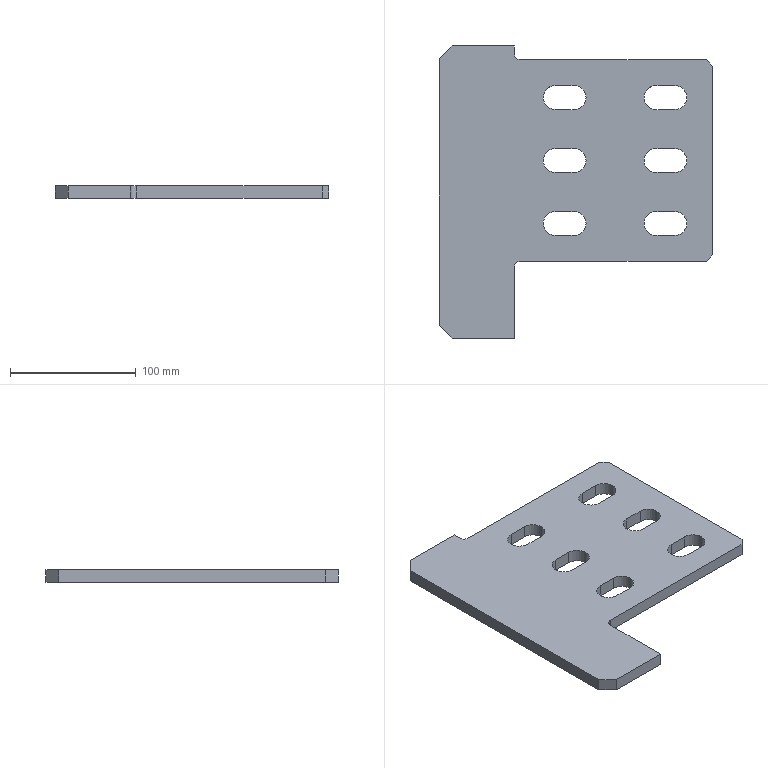Part | STEP file | 筋Plate-250×125-200 | 1 solid | 46 faces | box 217 x 232 x 10 mm | volume 354786 mm3 | plane 26 | cylinder 20 | commonest cylinder face diameters 19 x18 10 x2